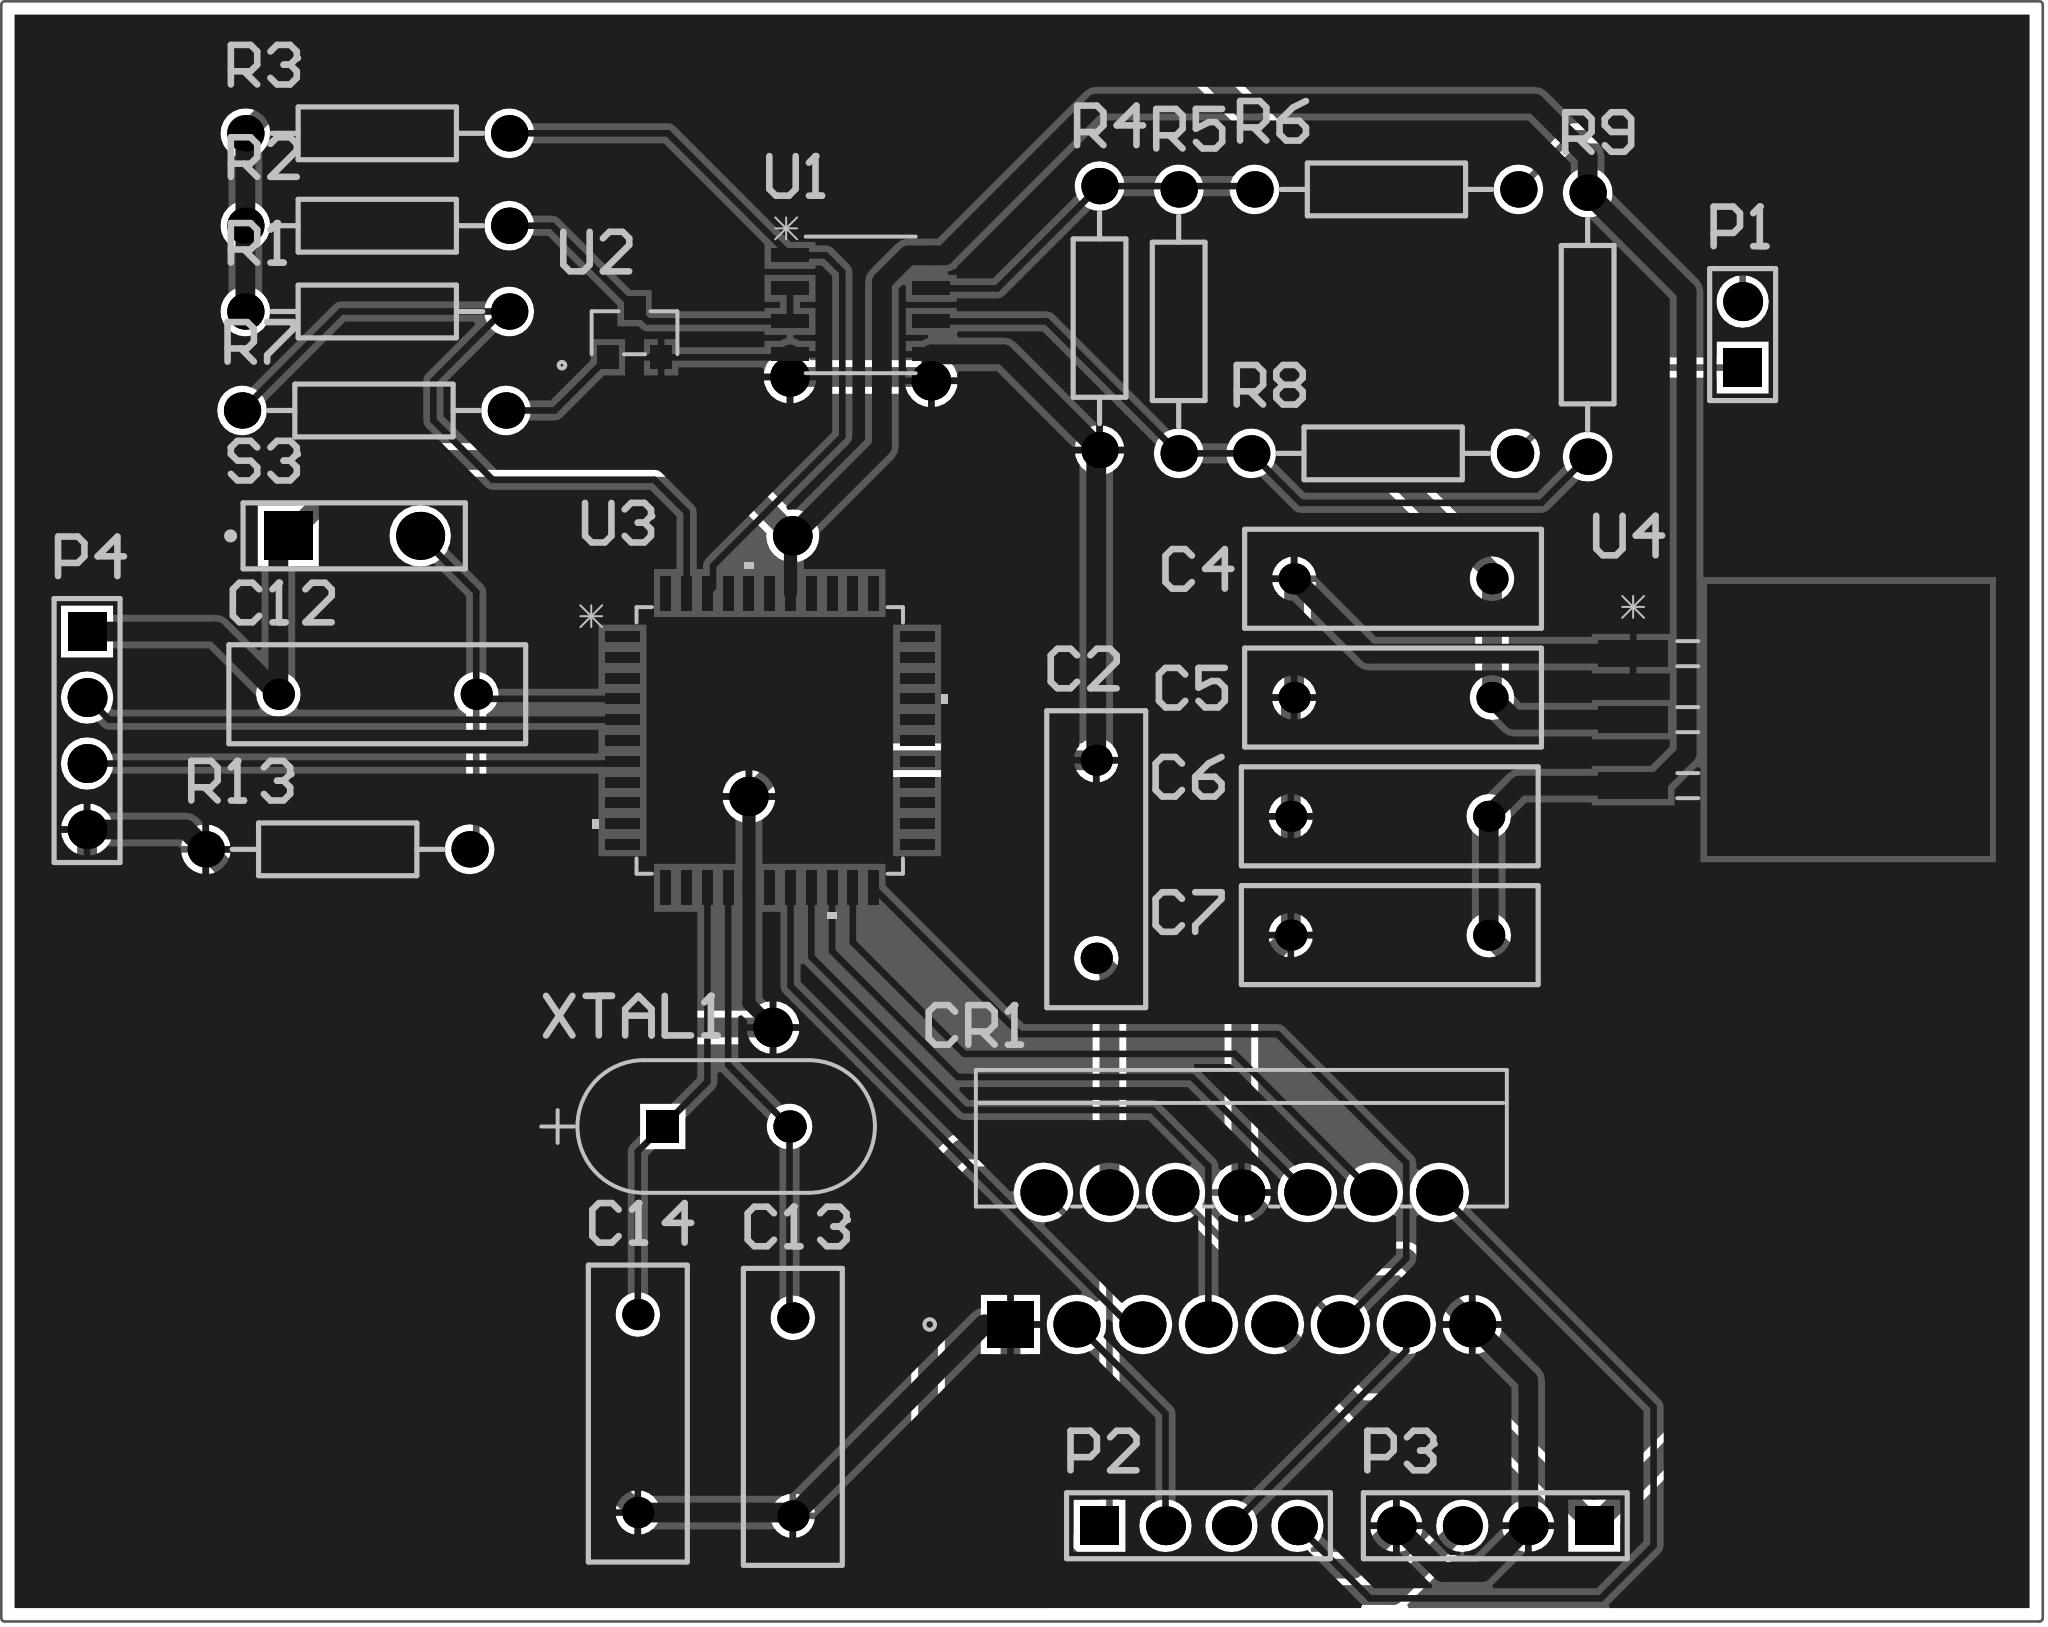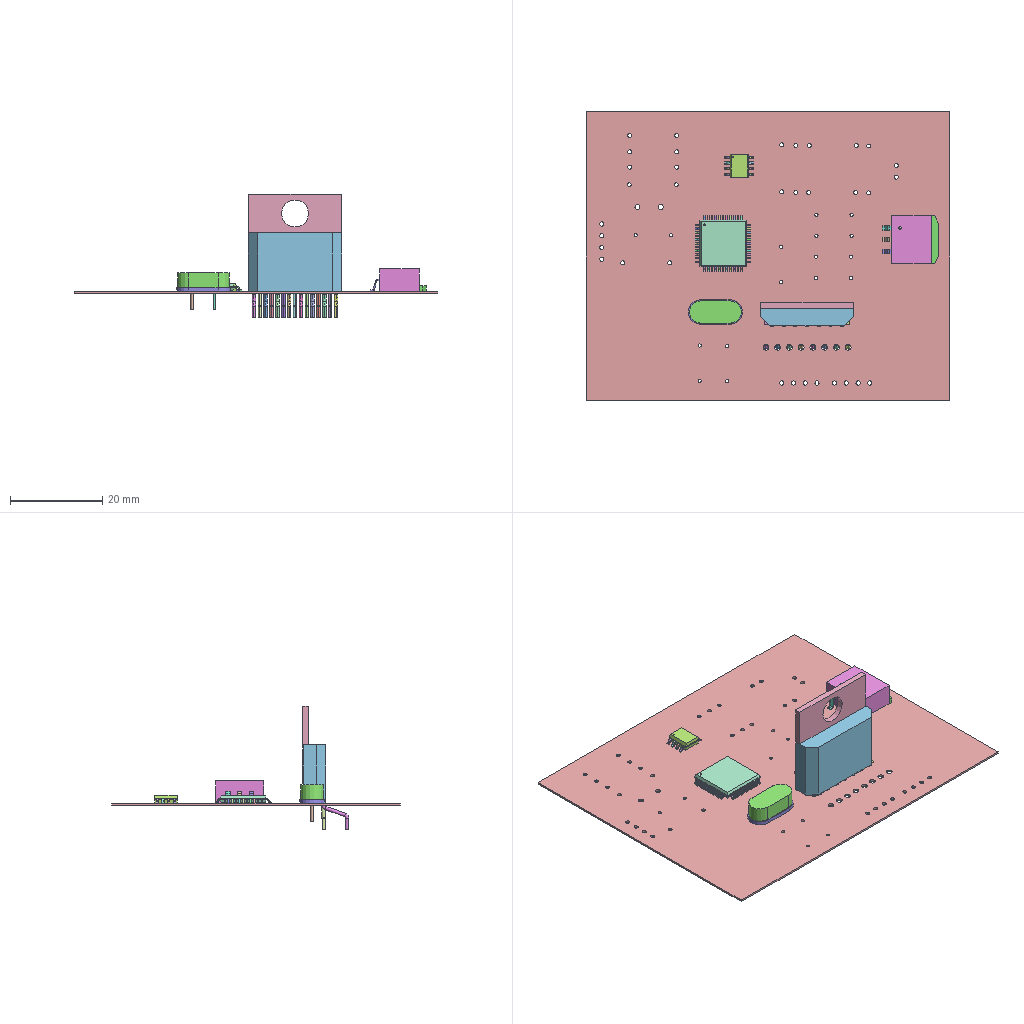Circuit board layout | Altium Designer | box 78.6 x 62.4 x 26.8 mm
Part placement:
Designator,Comment,Layer,Footprint,Center-X(mm),Center-Y(mm),Rotation
P1,Header 2,TopLayer,HDR1X2,122.047,90.043,90
R6,Res2,TopLayer,AXIAL-0.4,108.331,95.631,360
R2,Res2,TopLayer,AXIAL-0.4,69.469,94.234,180
R8,Res2,TopLayer,AXIAL-0.4,108.204,85.471,360
R7,Res2,TopLayer,AXIAL-0.4,69.342,87.122,360
R1,Res2,TopLayer,AXIAL-0.4,69.469,90.932,180
R4,Res2,TopLayer,AXIAL-0.4,97.282,90.678,270
R5,Res2,TopLayer,AXIAL-0.4,100.33,90.551,90
R3,Res2,TopLayer,AXIAL-0.4,69.469,97.79,180
R9,Res2,TopLayer,AXIAL-0.4,116.078,90.424,270
C2,Cap,TopLayer,RAD-0.3,97.155,69.85,270
P2,Header 4,TopLayer,HDR1X4,101.092,44.196,360
R13,Res2,TopLayer,AXIAL-0.4,67.945,70.231,360
C4,Cap,TopLayer,RAD-0.3,108.585,80.645,360
C7,Cap,TopLayer,RAD-0.3,108.458,66.929,360
C6,Cap,TopLayer,RAD-0.3,108.458,71.501,360
C5,Cap,TopLayer,RAD-0.3,108.585,76.073,360
U1,MAX485CSA+,TopLayer,21-0041B_8_MXM,88.084,91.186,0
U3,STC12C5A60S2-35I-LQFP44,TopLayer,LQFP44_STC89_STC_SCM,84.582,74.422,360
U4,AMS1117-3.3,TopLayer,TS3B_TEX,121.971,75.222,270
U2,MMBT3904-7-F,TopLayer,SOT-23_1_DIO,79.375,90.114,360
C12,Cap,TopLayer,RAD-0.3,69.469,76.2,360
C13,Cap,TopLayer,RAD-0.3,85.471,48.387,90
C14,Cap,TopLayer,RAD-0.3,79.502,48.514,90
P4,Header 4,TopLayer,HDR1X4,58.293,74.803,270
S3,SW-PB,TopLayer,SPST-2,68.58,82.296,360
CR1,L298N,TopLayer,Multiwatt15_V_STM,102.743,54.483,360
P3,Header 4,TopLayer,HDR1X4,112.522,44.196,180
XTAL1,HC49S-11.059-30-50-70-30-ATF,TopLayer,XTAL_HC49S_MTC,82.904,59.563,360